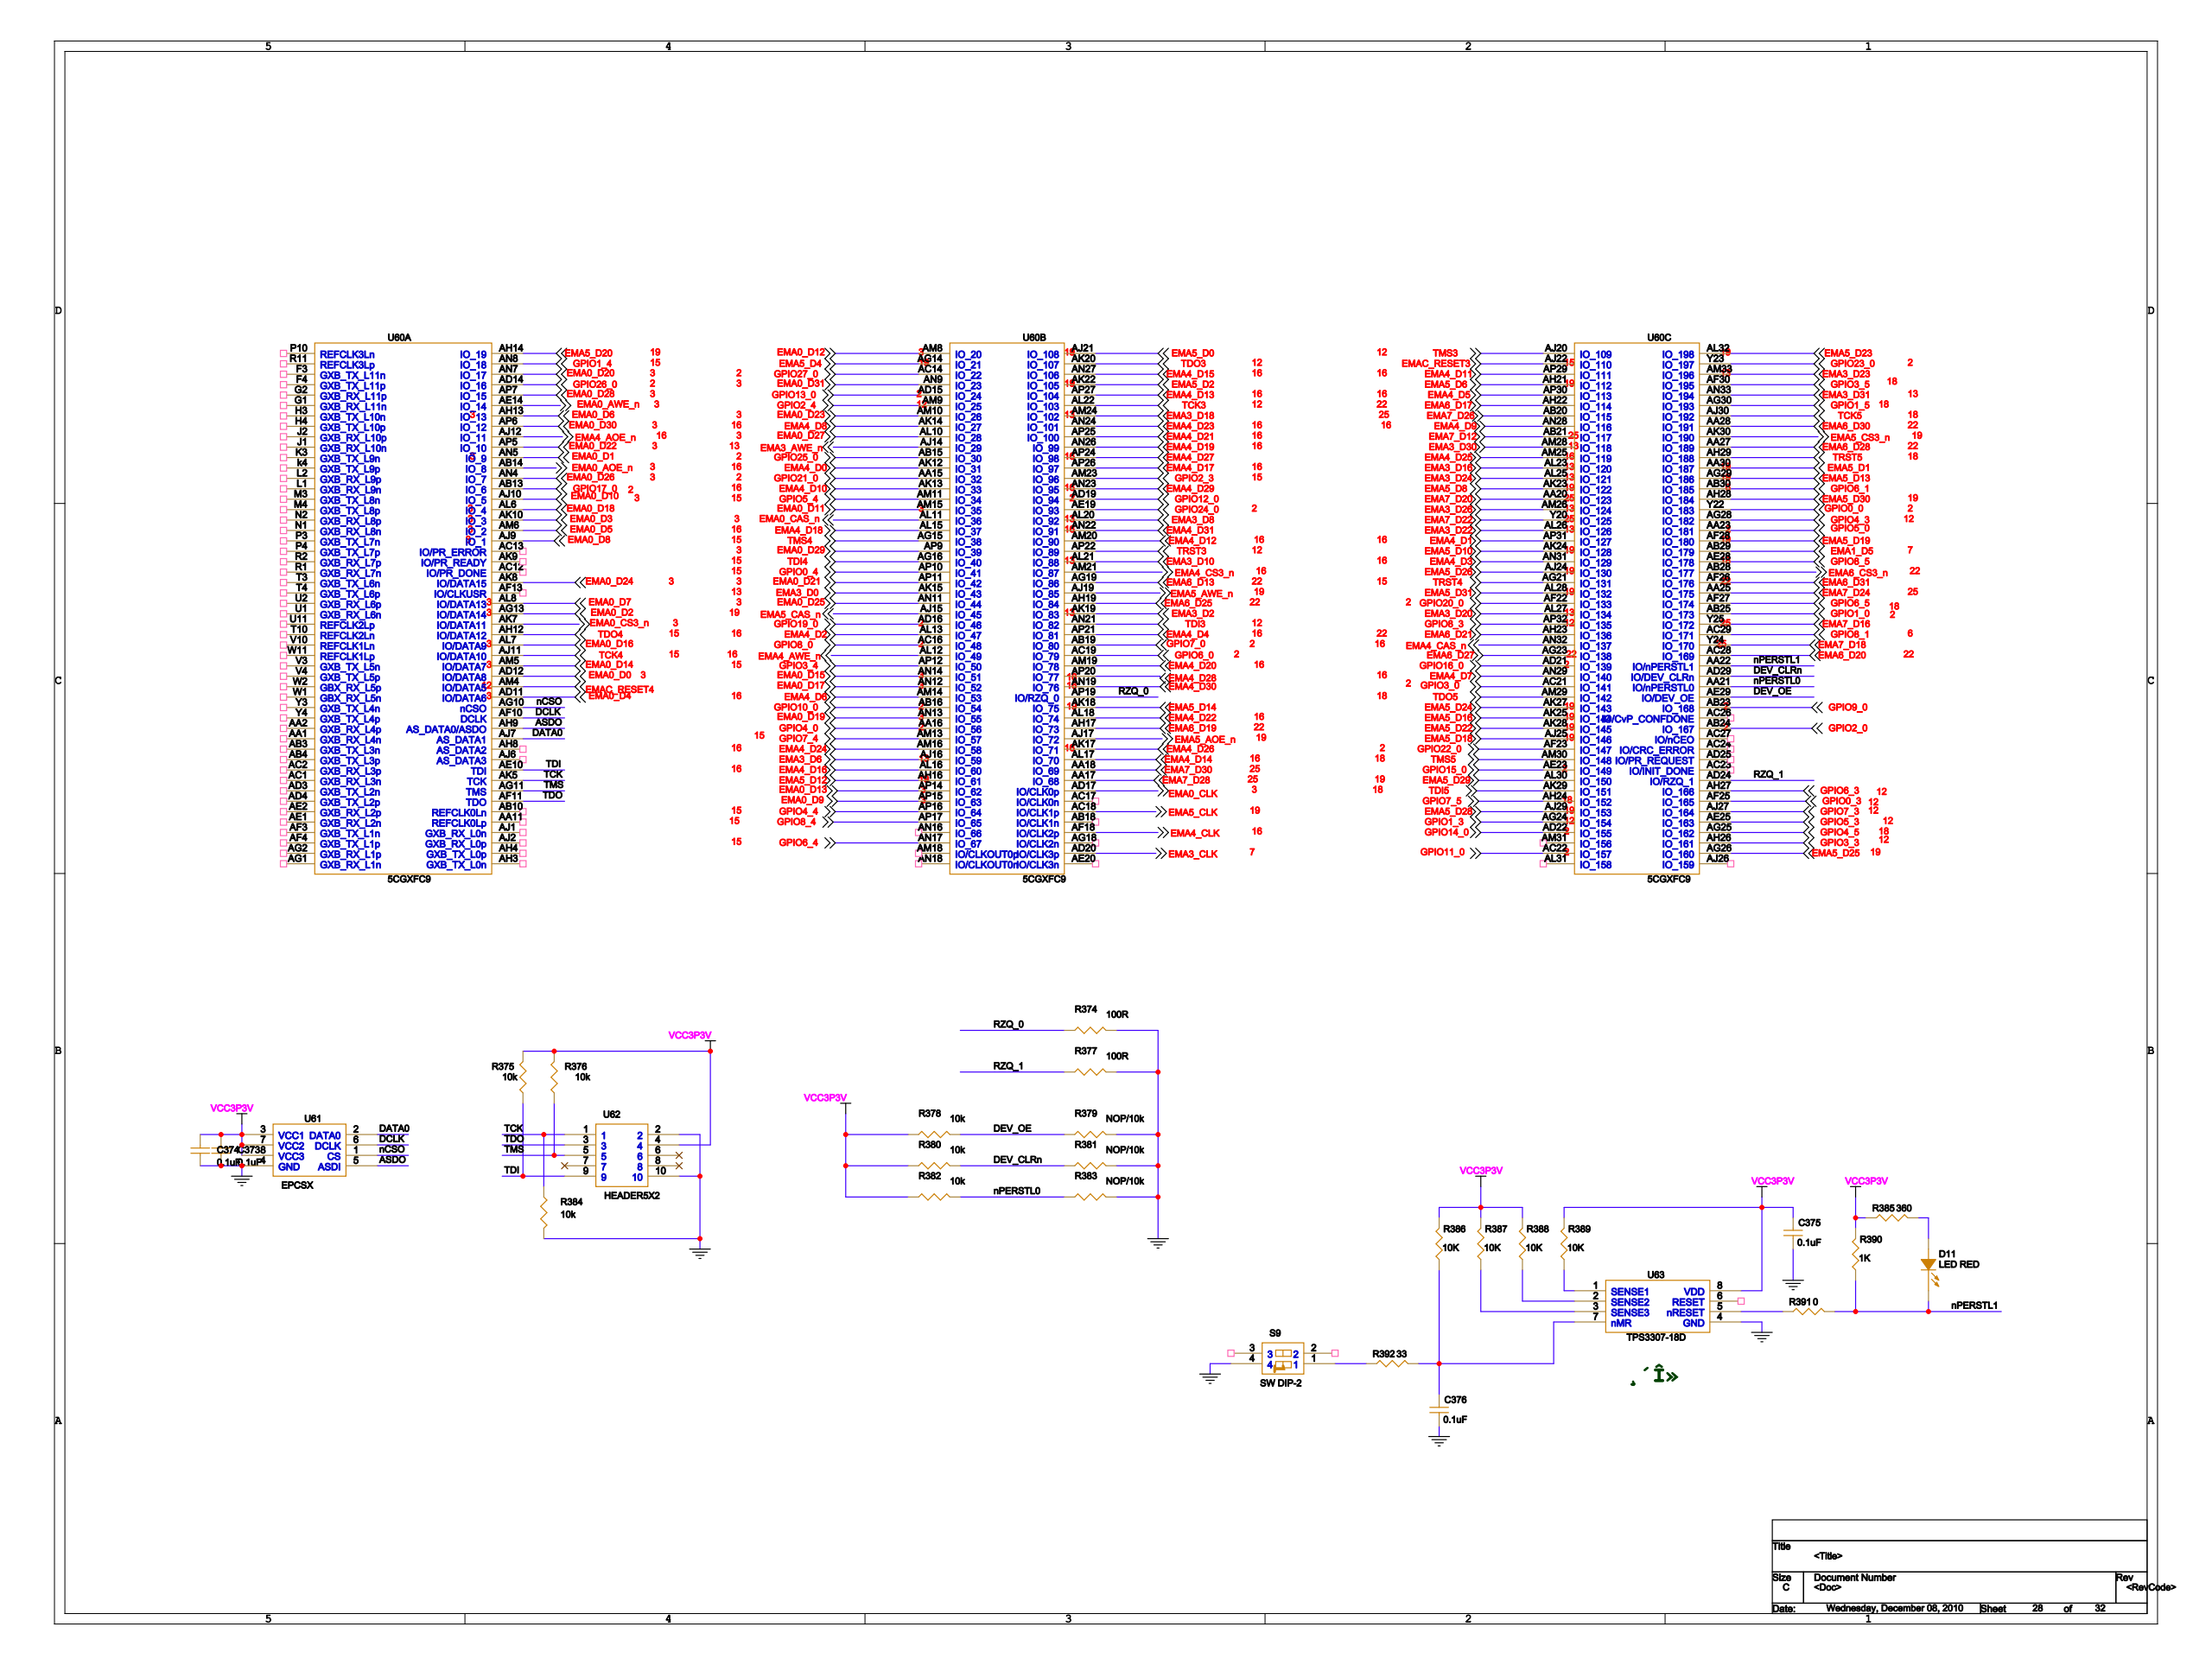Circuit board | Cadence Allegro | 1001 parts | 1318 nets | one sheet of the schematic
Parts on this sheet (reference | value | footprint):
C373 | 0.1uF | 0603
C374 | 0.1uF | 0603
C375 | 0.1uF | 0603
C376 | 0.1uF | 0603
R374 | 100R | 0603
R375 | 10K | 0603
R376 | 10K | 0603
R377 | 100R | 0603
R378 | 10K | 0603
R379 | NOP/10k | 0603
R380 | 10K | 0603
R381 | NOP/10k | 0603
R382 | 10K | 0603
R383 | NOP/10k | 0603
R384 | 10K | 0603
R385 | 360 | 0603
R386 | 10K | 0603
R387 | 10K | 0603
R388 | 10K | 0603
R389 | 10K | 0603
R390 | 1K | 0603
R391 | 0 | 0603
R392 | 33 | 0603
S9 | SW DIP-2 | SW_4
U1 | SoC_HTC_01 | L529_XIN
U2 | MT48LC32M16 | TSOP54
U11 | MT48LC32M16 | TSOP54
U60 | 5CGXFC9 | FBGA1152
U61 | EPCSX | SO-8
U62 | HEADER5X2 | CON2X5
U63 | TPS3307-18D | SO8
Nets of these parts (net: part-pin ...):
ASDO: U61-5 U60-AH9
DATA0: U61-2 U60-AJ7
DCLK: U61-6 U60-AF10
GPIO17_0: U60-AB13
GPIO26_0: U60-AD14
EMA0_D6: U60-AH13
EMA5_D20: U60-AH14
EMA0_D10: U60-AJ10
EMA0_D8: U60-AJ9
EMA0_D3: U60-AK10
EMA0_D18: U60-AL6
EMA0_D5: U1-AB15 U60-AM6
EMA0_D26: U60-AN4
EMA0_D1: U1-AB14 U60-AN5
EMA0_D20: U60-AN7
GPIO1_4: U60-AN8
EMA0_D22: U60-AP5
EMA0_D30: U60-AP6
EMA0_D28: U60-AP7
TCK4: U60-AJ11
TDO4: U60-AH12
EMA0_D7: U1-AC16 U60-AL8
EMA0_D2: U60-AG13
EMA0_D24: U60-AK8
EMAC_RESET4: U60-AM4
EMA0_D4: U60-AD11
EMA0_D14: U60-AM5
EMA0_D0: U60-AD12
EMA0_D16: U60-AL7
NCSO: U61-1 U60-AG10
TCK: R384-1 U62-1 U60-AK5
TDI: R375-1 U62-9 U60-AE10
TDO: U62-3 U60-AF11
TMS: R376-1 U62-5 U60-AG11
GPIO21_0: U60-AA15
GPIO4_0: U60-AA16
EMA7_D28: U60-AA17
EMA7_D30: U60-AA18
GPIO25_0: U60-AB15
GPIO10_0: U60-AB16
GPIO7_0: U60-AB19
GPIO27_0: U60-AC14
GPIO8_0: U60-AC16
GPIO6_0: U60-AC19
GPIO13_0: U60-AD15
GPIO19_0: U60-AD16
GPIO12_0: U60-AD19
GPIO24_0: U60-AE19
EMA5_D4: U60-AG14
TMS4: U60-AG15
TDI4: U60-AG16
EMA6_D13: U60-AG19
EMA5_D12: U60-AH16
EMA6_D19: U60-AH17
EMA6_D25: U60-AH19
EMA3_D6: U60-AJ16
EMA5_D0: U60-AJ21
EMA4_D0: U60-AK12
EMA4_D10: U60-AK13
EMA4_D8: U60-AK14
EMA3_D0: U60-AK15
EMA4_D26: U60-AK17
EMA5_D14: U60-AK18
EMA3_D2: U60-AK19
TDO3: U60-AK20
EMA5_D2: U60-AK22
EMA0_D27: U1-AB20 U60-AL10
EMA4_D2: U60-AL13
EMA4_D18: U60-AL15
EMA4_D16: U60-AL16
EMA4_D14: U60-AL17
EMA4_D22: U60-AL18
EMA3_D8: U60-AL20
EMA3_D10: U60-AL21
TCK3: U60-AL22
EMA0_D23: U1-AC21 U60-AM10
GPIO5_4: U60-AM11
GPIO7_4: U60-AM13
EMA4_D6: U60-AM14
EMA0_D11: U1-AB16 U60-AM15
EMA4_D24: U60-AM16
EMA4_D20: U60-AM19
EMA4_D12: U60-AM20
GPIO2_3: U60-AM23
EMA3_D18: U60-AM24
EMA0_D12: U60-AM8
GPIO2_4: U60-AM9
EMA0_D25: U1-AB19 U60-AN11
EMA0_D17: U1-AC19 U60-AN12
EMA0_D19: U1-AB18 U60-AN13
EMA0_D15: U60-AN14
GPIO6_4: U60-AN17
EMA4_D30: U60-AN19
TDI3: U60-AN21
EMA4_D31: U60-AN22
EMA4_D29: U60-AN23
EMA4_D23: U60-AN24
EMA4_D19: U60-AN26
EMA4_D15: U60-AN27
EMA0_D31: U60-AN9
GPIO0_4: U60-AP10
EMA0_D21: U60-AP11
GPIO3_4: U60-AP12
EMA0_D13: U1-AC18 U60-AP14
EMA0_D9: U1-AC17 U60-AP15
GPIO4_4: U60-AP16
GPIO8_4: U60-AP17
EMA4_D28: U60-AP20
EMA4_D4: U60-AP21
TRST3: U60-AP22
EMA4_D27: U60-AP24
EMA4_D21: U60-AP25
EMA4_D17: U60-AP26
EMA4_D13: U60-AP27
EMA0_D29: U1-AB21 U60-AP9
EMA0_CLK: U60-AD17
EMA5_CLK: U60-AC18
EMA4_CLK: U60-AF18
EMA3_CLK: U60-AD20
RZQ_0: R374-1 U60-AP19
EMA7_D20: U60-AA20
GPIO5_0: U60-AA23
EMA7_D24: U60-AA25
EMA6_D28: U60-AA27
EMA6_D30: U60-AA28
EMA5_D1: U60-AA30
EMA7_D26: U60-AB20
EMA7_D12: U60-AB21
GPIO9_0: U60-AB23
GPIO2_0: U60-AB24
GPIO1_0: U60-AB25
EMA1_D5: U60-AB29
GPIO6_1: U60-AB30
GPIO3_0: U60-AC21
GPIO11_0: U60-AC22
EMA6_D20: U60-AC28
GPIO8_1: U60-AC29
GPIO16_0: U60-AD21
GPIO14_0: U60-AD22
GPIO15_0: U60-AE23
GPIO5_3: U60-AE25
GPIO8_5: U60-AE28
GPIO20_0: U60-AF22
GPIO22_0: U60-AF23
GPIO0_3: U60-AF25
EMA6_D31: U60-AF26
GPIO6_5: U60-AF27
EMA5_D19: U60-AF28
GPIO3_5: U60-AF30
TRST4: U60-AG21
EMA6_D27: U60-AG23
GPIO1_3: U60-AG24
GPIO4_5: U60-AG25
EMA5_D25: U60-AG26
GPIO4_3: U60-AG28
EMA5_D13: U60-AG29
GPIO1_5: U60-AG30
EMA5_D6: U60-AH21
EMA6_D17: U60-AH22
EMA6_D21: U60-AH23
GPIO7_5: U60-AH24
GPIO3_3: U60-AH26
GPIO6_3: U60-AH27
EMA5_D30: U60-AH28
TRST5: U60-AH29
TMS3: U60-AJ20
EMAC_RESET3: U60-AJ22
EMA5_D26: U60-AJ24
EMA5_D18: U60-AJ25
GPIO7_3: U60-AJ27
EMA5_D28: U60-AJ29
TCK5: U60-AJ30
EMA5_D8: U60-AK23
EMA5_D10: U60-AK24
EMA5_D16: U60-AK25
EMA5_D24: U60-AK27
EMA5_D22: U60-AK28
TDI5: U60-AK29
EMA3_D16: U60-AL23
EMA3_D24: U60-AL25
EMA3_D22: U60-AL26
EMA3_D20: U60-AL27
EMA5_D31: U60-AL28
EMA5_D29: U60-AL30
EMA5_D23: U60-AL32
EMA4_D25: U60-AM25
EMA3_D26: U60-AM26
EMA3_D30: U60-AM28
TDO5: U60-AM29
TMS5: U60-AM30
EMA3_D23: U60-AM33
EMA4_D9: U60-AN28
EMA4_D7: U60-AN29
EMA4_D3: U60-AN31
EMA3_D31: U60-AN33
EMA4_D11: U60-AP29
EMA4_D5: U60-AP30
EMA4_D1: U60-AP31
GPIO8_3: U60-AP32
EMA7_D22: U60-Y20
GPIO0_0: U60-Y22
GPIO23_0: U60-Y23
EMA7_D18: U60-Y24
EMA7_D16: U60-Y25
DEV_CLRN: R380-2 R381-1 U60-AD29
DEV_OE: R378-2 R379-1 U60-AE29
NPERSTL0: R382-2 R383-1 U60-AA21
NPERSTL1: R390-1 R391-2 U60-AA22
RZQ_1: R377-1 U60-AD24
GND: C373-1 C374-1 C375-2 C376-2 R374-2 R377-2 R379-2 R381-2 R383-2 R384-2 S9-4 U61-4 U62-2 U62-10 U63-4 U1-AA11 U1-AA16 U1-AA18 U1-AB3 U1-F4 U1-H4 U1-M3 U1-N2 U1-P3 U1-T4 U1-T10 U1-V10 U2-6 U2-12 U2-28 U11-6 U11-12 U11-28
VCC3P3V: C373-2 C374-2 C375-1 R375-2 R376-2 R378-1 R380-1 R382-1 R385-1 R386-2 R387-2 R388-2 R389-2 R390-2 U61-3 U61-7 U61-8 U62-4 U63-8 U1-G1 U1-G2 U1-H3 U1-P4 U1-T3 U2-1 U2-3 U2-9 U11-1 U11-3 U11-9
N17701522: C376-1 R386-1 R392-2 U63-7
N17701532: R385-2
N17701540: R387-1 U63-3
N17701516: R388-1 U63-2
N17701548: R389-1 U63-1
N17701546: R391-1 U63-5
N17701574: R392-1 S9-1